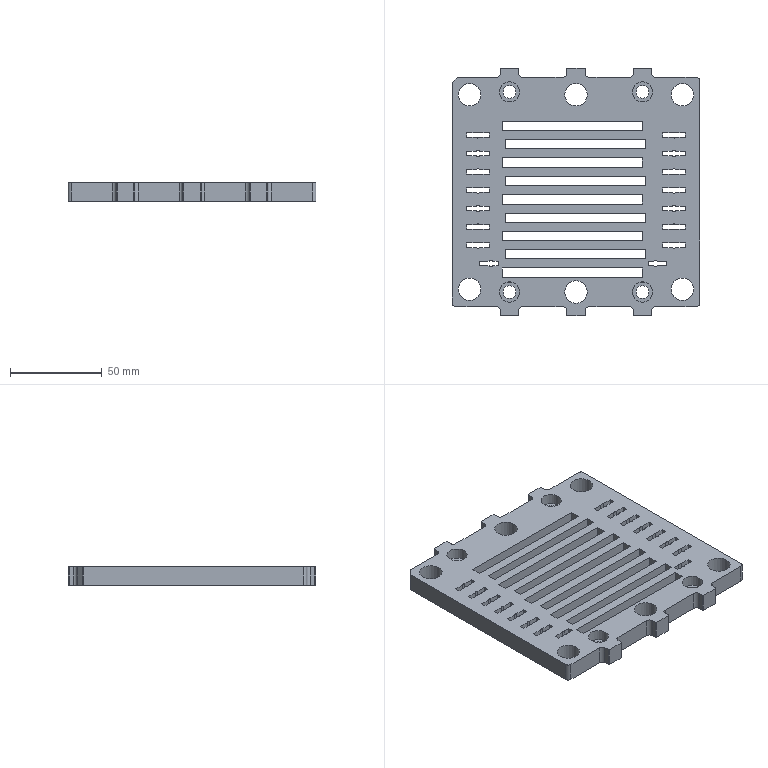Part | STEP file | 200 mesh_id2110 | 1 solid | 290 faces | box 135.01 x 135.01 x 10 mm | volume 121215 mm3 | plane 191 | cylinder 99 | commonest cylinder face diameters 3.2 x32 6 x24 1.01 x14 3.99 x12 12.3 x6 7 x4